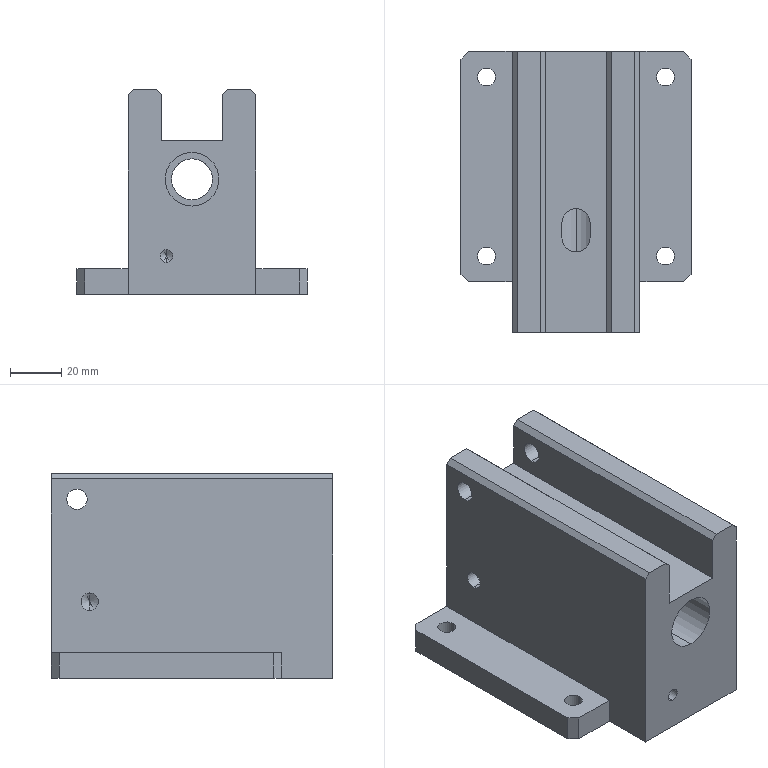Part | STEP file | 0217_201_Base | 1 solid | 60 faces | box 90 x 110 x 80 mm | volume 389355 mm3 | plane 28 | cylinder 26 | cone 6 | commonest cylinder face diameters 7 x8 6.8 x4 8 x4 21 x4 5 x2 11 x2